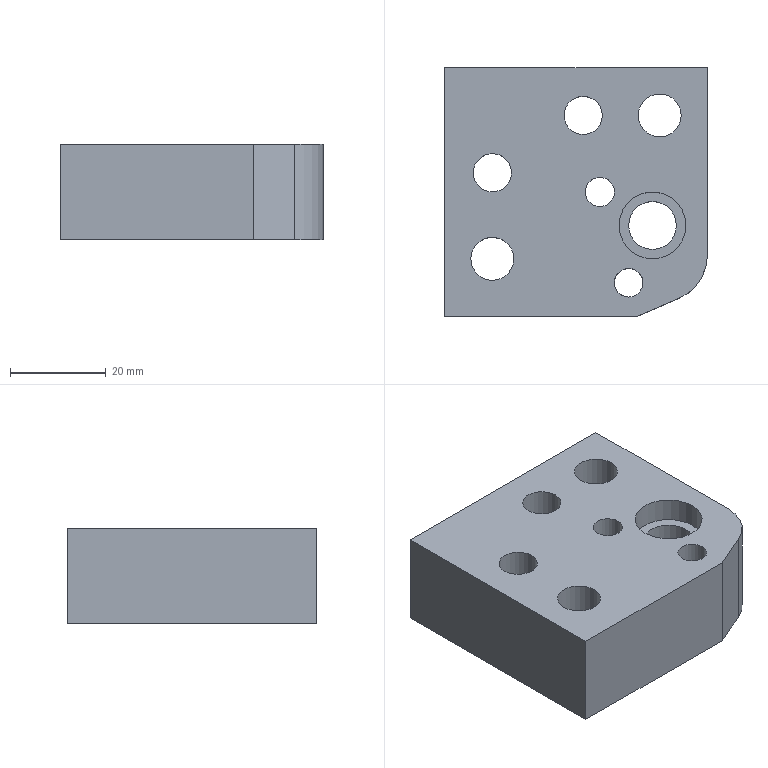Part | STEP file | 411_id2394_x_t | 1 solid | 25 faces | box 55 x 52 x 20 mm | volume 46099 mm3 | cylinder 13 | plane 12 | commonest cylinder face diameters 10 x3 14 x3 8 x2 9 x2 6 x1 6.1 x1